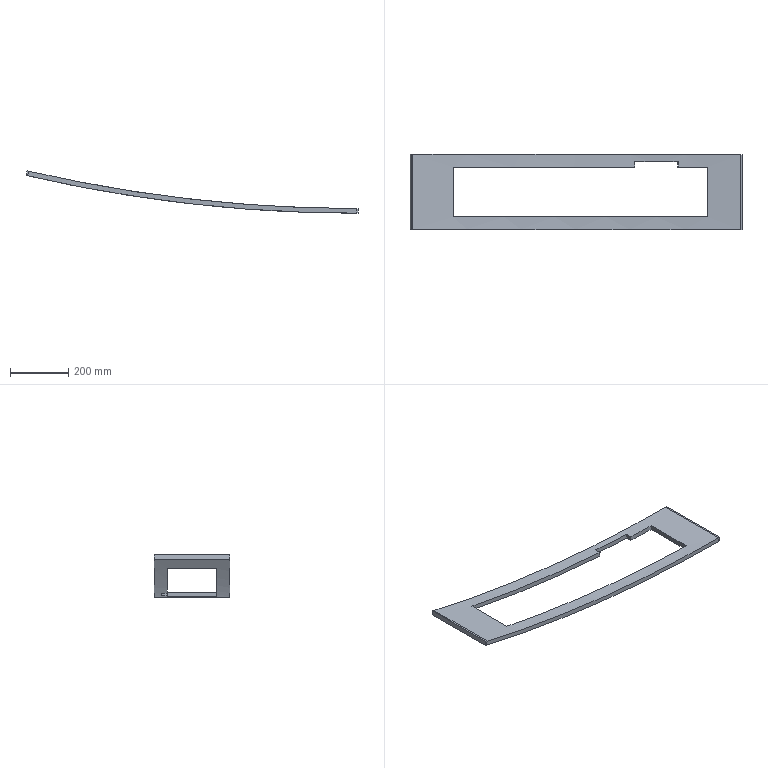Part | SolidWorks | features FlatPattern 1, SM3dBend 1, SMBaseFlange 1, SheetMetal 1 | 1 solid | 22 faces | box 1142 x 258 x 145.694 mm | volume 2305600 mm3 | plane 20 | cylinder 2 | commonest cylinder face diameters 10020 x1 10052 x1
STEP:
#1=CARTESIAN_POINT('',(17.269,258.,128.406));
#2=VERTEX_POINT('',#1);
#3=CARTESIAN_POINT('',(11.69,258.,129.694));
#4=VERTEX_POINT('',#3);
#5=CARTESIAN_POINT('',(11.69,258.,129.694));
#6=DIRECTION('',(-0.9744,0.,0.225));
#7=VECTOR('',#6,1000.);
#8=LINE('',#5,#7);
#9=EDGE_CURVE('',#2,#4,#8,.T.);
#10=ORIENTED_EDGE('',*,*,#9,.F.);
#11=CARTESIAN_POINT('',(13.67,258.,112.816));
#12=VERTEX_POINT('',#11);
#13=CARTESIAN_POINT('',(13.67,258.,112.816));
#14=DIRECTION('',(-0.225,0.,-0.9744));
#15=VECTOR('',#14,1000.);
#16=LINE('',#13,#15);
#17=EDGE_CURVE('',#2,#12,#16,.T.);
#18=ORIENTED_EDGE('',*,*,#17,.T.);
#19=CARTESIAN_POINT('',(8.091,258.,114.104));
#20=VERTEX_POINT('',#19);
#21=CARTESIAN_POINT('',(8.091,258.,114.104));
#22=DIRECTION('',(-0.9744,0.,0.225));
#23=VECTOR('',#22,1000.);
#24=LINE('',#21,#23);
#25=EDGE_CURVE('',#12,#20,#24,.T.);
#26=ORIENTED_EDGE('',*,*,#25,.T.);
#27=CARTESIAN_POINT('',(8.091,258.,114.104));
#28=DIRECTION('',(0.225,0.,0.9744));
#29=VECTOR('',#28,1000.);
#30=LINE('',#27,#29);
#31=EDGE_CURVE('',#20,#4,#30,.T.);
#32=ORIENTED_EDGE('',*,*,#31,.T.);
#33=EDGE_LOOP('',(#10,#18,#26,#32));
#34=FACE_OUTER_BOUND('',#33,.T.);
#35=CARTESIAN_POINT('',(8.091,258.,114.104));
#36=DIRECTION('',(0.,1.,0.));
#37=DIRECTION('',(0.225,0.,0.9744));
#38=AXIS2_PLACEMENT_3D('',#35,#36,#37);
#39=PLANE('',#38);
#40=ADVANCED_FACE('',(#34),#39,.T.);
#41=CARTESIAN_POINT('',(8.091,0.,114.104));
#42=VERTEX_POINT('',#41);
#43=CARTESIAN_POINT('',(13.67,0.,112.816));
#44=VERTEX_POINT('',#43);
#45=CARTESIAN_POINT('',(8.091,0.,114.104));
#46=DIRECTION('',(0.9744,0.,-0.225));
#47=VECTOR('',#46,1000.);
#48=LINE('',#45,#47);
#49=EDGE_CURVE('',#42,#44,#48,.T.);
#50=ORIENTED_EDGE('',*,*,#49,.T.);
#51=CARTESIAN_POINT('',(17.269,0.,128.406));
#52=VERTEX_POINT('',#51);
#53=CARTESIAN_POINT('',(13.67,0.,112.816));
#54=DIRECTION('',(0.225,0.,0.9744));
#55=VECTOR('',#54,1000.);
#56=LINE('',#53,#55);
#57=EDGE_CURVE('',#44,#52,#56,.T.);
#58=ORIENTED_EDGE('',*,*,#57,.T.);
#59=CARTESIAN_POINT('',(11.69,0.,129.694));
#60=VERTEX_POINT('',#59);
#61=CARTESIAN_POINT('',(11.69,0.,129.694));
#62=DIRECTION('',(0.9744,0.,-0.225));
#63=VECTOR('',#62,1000.);
#64=LINE('',#61,#63);
#65=EDGE_CURVE('',#60,#52,#64,.T.);
#66=ORIENTED_EDGE('',*,*,#65,.F.);
#67=CARTESIAN_POINT('',(8.091,0.,114.104));
#68=DIRECTION('',(0.225,0.,0.9744));
#69=VECTOR('',#68,1000.);
#70=LINE('',#67,#69);
#71=EDGE_CURVE('',#42,#60,#70,.T.);
#72=ORIENTED_EDGE('',*,*,#71,.F.);
#73=EDGE_LOOP('',(#50,#58,#66,#72));
#74=FACE_OUTER_BOUND('',#73,.T.);
#75=CARTESIAN_POINT('',(8.091,0.,114.104));
#76=DIRECTION('',(0.,-1.,0.));
#77=DIRECTION('',(-0.225,0.,-0.9744));
#78=AXIS2_PLACEMENT_3D('',#75,#76,#77);
#79=PLANE('',#78);
#80=ADVANCED_FACE('',(#74),#79,.T.);
#81=ORIENTED_EDGE('',*,*,#25,.F.);
#82=CARTESIAN_POINT('',(13.67,258.,112.816));
#83=DIRECTION('',(0.,-1.,0.));
#84=VECTOR('',#83,1000.);
#85=LINE('',#82,#84);
#86=EDGE_CURVE('',#12,#44,#85,.T.);
#87=ORIENTED_EDGE('',*,*,#86,.T.);
#88=ORIENTED_EDGE('',*,*,#49,.F.);
#89=CARTESIAN_POINT('',(8.091,0.,114.104));
#90=DIRECTION('',(0.,-1.,0.));
#91=VECTOR('',#90,1000.);
#92=LINE('',#89,#91);
#93=EDGE_CURVE('',#20,#42,#92,.T.);
#94=ORIENTED_EDGE('',*,*,#93,.F.);
#95=EDGE_LOOP('',(#81,#87,#88,#94));
#96=FACE_OUTER_BOUND('',#95,.T.);
#97=CARTESIAN_POINT('',(8.091,258.,114.104));
#98=DIRECTION('',(-0.225,0.,-0.9744));
#99=DIRECTION('',(-0.9744,0.,0.225));
#100=AXIS2_PLACEMENT_3D('',#97,#98,#99);
#101=PLANE('',#100);
#102=ADVANCED_FACE('',(#96),#101,.T.);
#103=CARTESIAN_POINT('',(11.69,0.,129.694));
#104=DIRECTION('',(0.,-1.,0.));
#105=VECTOR('',#104,1000.);
#106=LINE('',#103,#105);
#107=EDGE_CURVE('',#4,#60,#106,.T.);
#108=ORIENTED_EDGE('',*,*,#107,.F.);
#109=ORIENTED_EDGE('',*,*,#31,.F.);
#110=ORIENTED_EDGE('',*,*,#93,.T.);
#111=ORIENTED_EDGE('',*,*,#71,.T.);
#112=EDGE_LOOP('',(#108,#109,#110,#111));
#113=FACE_OUTER_BOUND('',#112,.T.);
#114=CARTESIAN_POINT('',(8.091,0.,114.104));
#115=DIRECTION('',(-0.9744,0.,0.225));
#116=DIRECTION('',(0.225,0.,0.9744));
#117=AXIS2_PLACEMENT_3D('',#114,#115,#116);
#118=PLANE('',#117);
#119=ADVANCED_FACE('',(#113),#118,.T.);
#120=CARTESIAN_POINT('',(17.269,258.,128.406));
#121=DIRECTION('',(0.,-1.,0.));
#122=VECTOR('',#121,1000.);
#123=LINE('',#120,#122);
#124=EDGE_CURVE('',#2,#52,#123,.T.);
#125=ORIENTED_EDGE('',*,*,#124,.F.);
#126=ORIENTED_EDGE('',*,*,#9,.T.);
#127=ORIENTED_EDGE('',*,*,#107,.T.);
#128=ORIENTED_EDGE('',*,*,#65,.T.);
#129=EDGE_LOOP('',(#125,#126,#127,#128));
#130=FACE_OUTER_BOUND('',#129,.T.);
#131=CARTESIAN_POINT('',(11.69,258.,129.694));
#132=DIRECTION('',(-0.225,0.,-0.9744));
#133=DIRECTION('',(-0.9744,0.,0.225));
#134=AXIS2_PLACEMENT_3D('',#131,#132,#133);
#135=PLANE('',#134);
#136=ADVANCED_FACE('',(#130),#135,.F.);
#137=CARTESIAN_POINT('',(1150.,0.,0.));
#138=VERTEX_POINT('',#137);
#139=CARTESIAN_POINT('',(1150.,258.,0.));
#140=VERTEX_POINT('',#139);
#141=CARTESIAN_POINT('',(1150.,0.,0.));
#142=DIRECTION('',(0.,1.,0.));
#143=VECTOR('',#142,1000.);
#144=LINE('',#141,#143);
#145=EDGE_CURVE('',#138,#140,#144,.T.);
#146=ORIENTED_EDGE('',*,*,#145,.F.);
#147=CARTESIAN_POINT('',(1150.,0.,-16.));
#148=VERTEX_POINT('',#147);
#149=CARTESIAN_POINT('',(1150.,0.,-16.));
#150=DIRECTION('',(0.,0.,1.));
#151=VECTOR('',#150,1000.);
#152=LINE('',#149,#151);
#153=EDGE_CURVE('',#148,#138,#152,.T.);
#154=ORIENTED_EDGE('',*,*,#153,.F.);
#155=CARTESIAN_POINT('',(1150.,258.,-16.));
#156=VERTEX_POINT('',#155);
#157=CARTESIAN_POINT('',(1150.,0.,-16.));
#158=DIRECTION('',(0.,1.,0.));
#159=VECTOR('',#158,1000.);
#160=LINE('',#157,#159);
#161=EDGE_CURVE('',#148,#156,#160,.T.);
#162=ORIENTED_EDGE('',*,*,#161,.T.);
#163=CARTESIAN_POINT('',(1150.,258.,-16.));
#164=DIRECTION('',(0.,0.,1.));
#165=VECTOR('',#164,1000.);
#166=LINE('',#163,#165);
#167=EDGE_CURVE('',#156,#140,#166,.T.);
#168=ORIENTED_EDGE('',*,*,#167,.T.);
#169=EDGE_LOOP('',(#146,#154,#162,#168));
#170=FACE_OUTER_BOUND('',#169,.T.);
#171=CARTESIAN_POINT('',(1150.,0.,-16.));
#172=DIRECTION('',(1.,0.,0.));
#173=DIRECTION('',(0.,0.,-1.));
#174=AXIS2_PLACEMENT_3D('',#171,#172,#173);
#175=PLANE('',#174);
#176=ADVANCED_FACE('',(#170),#175,.T.);
#177=CARTESIAN_POINT('',(1144.274,258.,-16.));
#178=VERTEX_POINT('',#177);
#179=CARTESIAN_POINT('',(1144.274,0.,-16.));
#180=VERTEX_POINT('',#179);
#181=CARTESIAN_POINT('',(1144.274,258.,-16.));
#182=DIRECTION('',(0.,-1.,0.));
#183=VECTOR('',#182,1000.);
#184=LINE('',#181,#183);
#185=EDGE_CURVE('',#178,#180,#184,.T.);
#186=ORIENTED_EDGE('',*,*,#185,.F.);
#187=CARTESIAN_POINT('',(0.,258.,-16.));
#188=DIRECTION('',(-1.,0.,0.));
#189=VECTOR('',#188,1000.);
#190=LINE('',#187,#189);
#191=EDGE_CURVE('',#156,#178,#190,.T.);
#192=ORIENTED_EDGE('',*,*,#191,.F.);
#193=ORIENTED_EDGE('',*,*,#161,.F.);
#194=CARTESIAN_POINT('',(0.,0.,-16.));
#195=DIRECTION('',(1.,0.,0.));
#196=VECTOR('',#195,1000.);
#197=LINE('',#194,#196);
#198=EDGE_CURVE('',#180,#148,#197,.T.);
#199=ORIENTED_EDGE('',*,*,#198,.F.);
#200=EDGE_LOOP('',(#186,#192,#193,#199));
#201=FACE_OUTER_BOUND('',#200,.T.);
#202=CARTESIAN_POINT('',(0.,258.,-16.));
#203=DIRECTION('',(0.,0.,-1.));
#204=DIRECTION('',(-1.,0.,0.));
#205=AXIS2_PLACEMENT_3D('',#202,#203,#204);
#206=PLANE('',#205);
#207=ADVANCED_FACE('',(#201),#206,.T.);
#208=CARTESIAN_POINT('',(1144.274,258.,0.));
#209=VERTEX_POINT('',#208);
#210=CARTESIAN_POINT('',(1144.274,258.,-16.));
#211=DIRECTION('',(0.,0.,-1.));
#212=VECTOR('',#211,1000.);
#213=LINE('',#210,#212);
#214=EDGE_CURVE('',#209,#178,#213,.T.);
#215=ORIENTED_EDGE('',*,*,#214,.F.);
#216=CARTESIAN_POINT('',(0.,258.,0.));
#217=DIRECTION('',(-1.,0.,0.));
#218=VECTOR('',#217,1000.);
#219=LINE('',#216,#218);
#220=EDGE_CURVE('',#140,#209,#219,.T.);
#221=ORIENTED_EDGE('',*,*,#220,.F.);
#222=ORIENTED_EDGE('',*,*,#167,.F.);
#223=ORIENTED_EDGE('',*,*,#191,.T.);
#224=EDGE_LOOP('',(#215,#221,#222,#223));
#225=FACE_OUTER_BOUND('',#224,.T.);
#226=CARTESIAN_POINT('',(0.,258.,-16.));
#227=DIRECTION('',(0.,1.,0.));
#228=DIRECTION('',(0.,0.,1.));
#229=AXIS2_PLACEMENT_3D('',#226,#227,#228);
#230=PLANE('',#229);
#231=ADVANCED_FACE('',(#225),#230,.T.);
#232=ORIENTED_EDGE('',*,*,#220,.T.);
#233=CARTESIAN_POINT('',(1144.274,0.,0.));
#234=VERTEX_POINT('',#233);
#235=CARTESIAN_POINT('',(1144.274,258.,0.));
#236=DIRECTION('',(0.,-1.,0.));
#237=VECTOR('',#236,1000.);
#238=LINE('',#235,#237);
#239=EDGE_CURVE('',#209,#234,#238,.T.);
#240=ORIENTED_EDGE('',*,*,#239,.T.);
#241=CARTESIAN_POINT('',(0.,0.,0.));
#242=DIRECTION('',(1.,0.,0.));
#243=VECTOR('',#242,1000.);
#244=LINE('',#241,#243);
#245=EDGE_CURVE('',#234,#138,#244,.T.);
#246=ORIENTED_EDGE('',*,*,#245,.T.);
#247=ORIENTED_EDGE('',*,*,#145,.T.);
#248=EDGE_LOOP('',(#232,#240,#246,#247));
#249=FACE_OUTER_BOUND('',#248,.T.);
#250=CARTESIAN_POINT('',(0.,258.,0.));
#251=DIRECTION('',(0.,0.,-1.));
#252=DIRECTION('',(-1.,0.,0.));
#253=AXIS2_PLACEMENT_3D('',#250,#251,#252);
#254=PLANE('',#253);
#255=ADVANCED_FACE('',(#249),#254,.F.);
#256=CARTESIAN_POINT('',(1144.274,0.,-16.));
#257=DIRECTION('',(0.,0.,1.));
#258=VECTOR('',#257,1000.);
#259=LINE('',#256,#258);
#260=EDGE_CURVE('',#180,#234,#259,.T.);
#261=ORIENTED_EDGE('',*,*,#260,.F.);
#262=ORIENTED_EDGE('',*,*,#198,.T.);
#263=ORIENTED_EDGE('',*,*,#153,.T.);
#264=ORIENTED_EDGE('',*,*,#245,.F.);
#265=EDGE_LOOP('',(#261,#262,#263,#264));
#266=FACE_OUTER_BOUND('',#265,.T.);
#267=CARTESIAN_POINT('',(0.,0.,-16.));
#268=DIRECTION('',(0.,-1.,0.));
#269=DIRECTION('',(0.,0.,-1.));
#270=AXIS2_PLACEMENT_3D('',#267,#268,#269);
#271=PLANE('',#270);
#272=ADVANCED_FACE('',(#266),#271,.T.);
#273=CARTESIAN_POINT('',(780.9,234.,13.195));
#274=VERTEX_POINT('',#273);
#275=CARTESIAN_POINT('',(779.74,234.,-2.763));
#276=VERTEX_POINT('',#275);
#277=CARTESIAN_POINT('',(779.74,234.,-2.763));
#278=DIRECTION('',(-0.07253,0.,-0.9974));
#279=VECTOR('',#278,1000.);
#280=LINE('',#277,#279);
#281=EDGE_CURVE('',#274,#276,#280,.T.);
#282=ORIENTED_EDGE('',*,*,#281,.F.);
#283=CARTESIAN_POINT('',(780.9,214.,13.195));
#284=VERTEX_POINT('',#283);
#285=CARTESIAN_POINT('',(780.9,-1038.524,13.195));
#286=DIRECTION('',(0.,-1.,0.));
#287=VECTOR('',#286,1000.);
#288=LINE('',#285,#287);
#289=EDGE_CURVE('',#274,#284,#288,.T.);
#290=ORIENTED_EDGE('',*,*,#289,.T.);
#291=CARTESIAN_POINT('',(779.74,214.,-2.763));
#292=VERTEX_POINT('',#291);
#293=CARTESIAN_POINT('',(779.74,214.,-2.763));
#294=DIRECTION('',(-0.07253,0.,-0.9974));
#295=VECTOR('',#294,1000.);
#296=LINE('',#293,#295);
#297=EDGE_CURVE('',#284,#292,#296,.T.);
#298=ORIENTED_EDGE('',*,*,#297,.T.);
#299=CARTESIAN_POINT('',(779.74,234.,-2.763));
#300=DIRECTION('',(0.,-1.,0.));
#301=VECTOR('',#300,1000.);
#302=LINE('',#299,#301);
#303=EDGE_CURVE('',#276,#292,#302,.T.);
#304=ORIENTED_EDGE('',*,*,#303,.F.);
#305=EDGE_LOOP('',(#282,#290,#298,#304));
#306=FACE_OUTER_BOUND('',#305,.T.);
#307=CARTESIAN_POINT('',(779.74,224.,-2.763));
#308=DIRECTION('',(0.9974,0.,-0.07253));
#309=DIRECTION('',(0.,-1.,0.));
#310=AXIS2_PLACEMENT_3D('',#307,#308,#309);
#311=PLANE('',#310);
#312=ADVANCED_FACE('',(#306),#311,.T.);
#313=ORIENTED_EDGE('',*,*,#297,.F.);
#314=CARTESIAN_POINT('',(158.068,214.,98.025));
#315=VERTEX_POINT('',#314);
#316=CARTESIAN_POINT('',(1144.274,214.,5010.));
#317=DIRECTION('',(0.,1.,0.));
#318=DIRECTION('',(0.,0.,1.));
#319=AXIS2_PLACEMENT_3D('',#316,#317,#318);
#320=CIRCLE('',#319,5010.);
#321=EDGE_CURVE('',#284,#315,#320,.T.);
#322=ORIENTED_EDGE('',*,*,#321,.T.);
#323=CARTESIAN_POINT('',(154.918,214.,82.338));
#324=VERTEX_POINT('',#323);
#325=CARTESIAN_POINT('',(154.918,214.,82.338));
#326=DIRECTION('',(-0.1968,0.,-0.9804));
#327=VECTOR('',#326,1000.);
#328=LINE('',#325,#327);
#329=EDGE_CURVE('',#315,#324,#328,.T.);
#330=ORIENTED_EDGE('',*,*,#329,.T.);
#331=CARTESIAN_POINT('',(1144.274,214.,5010.));
#332=DIRECTION('',(0.,1.,0.));
#333=DIRECTION('',(0.,0.,1.));
#334=AXIS2_PLACEMENT_3D('',#331,#332,#333);
#335=CIRCLE('',#334,5026.);
#336=EDGE_CURVE('',#292,#324,#335,.T.);
#337=ORIENTED_EDGE('',*,*,#336,.F.);
#338=EDGE_LOOP('',(#313,#322,#330,#337));
#339=FACE_OUTER_BOUND('',#338,.T.);
#340=CARTESIAN_POINT('',(1144.274,214.,5010.));
#341=DIRECTION('',(0.,-1.,0.));
#342=DIRECTION('',(0.,0.,-1.));
#343=AXIS2_PLACEMENT_3D('',#340,#341,#342);
#344=PLANE('',#343);
#345=ADVANCED_FACE('',(#339),#344,.T.);
#346=ORIENTED_EDGE('',*,*,#329,.F.);
#347=CARTESIAN_POINT('',(158.068,44.,98.025));
#348=VERTEX_POINT('',#347);
#349=CARTESIAN_POINT('',(158.068,-1038.524,98.025));
#350=DIRECTION('',(0.,-1.,0.));
#351=VECTOR('',#350,1000.);
#352=LINE('',#349,#351);
#353=EDGE_CURVE('',#315,#348,#352,.T.);
#354=ORIENTED_EDGE('',*,*,#353,.T.);
#355=CARTESIAN_POINT('',(154.918,44.,82.338));
#356=VERTEX_POINT('',#355);
#357=CARTESIAN_POINT('',(154.918,44.,82.338));
#358=DIRECTION('',(-0.1968,0.,-0.9804));
#359=VECTOR('',#358,1000.);
#360=LINE('',#357,#359);
#361=EDGE_CURVE('',#348,#356,#360,.T.);
#362=ORIENTED_EDGE('',*,*,#361,.T.);
#363=CARTESIAN_POINT('',(154.918,214.,82.338));
#364=DIRECTION('',(0.,-1.,0.));
#365=VECTOR('',#364,1000.);
#366=LINE('',#363,#365);
#367=EDGE_CURVE('',#324,#356,#366,.T.);
#368=ORIENTED_EDGE('',*,*,#367,.F.);
#369=EDGE_LOOP('',(#346,#354,#362,#368));
#370=FACE_OUTER_BOUND('',#369,.T.);
#371=CARTESIAN_POINT('',(154.918,129.,82.338));
#372=DIRECTION('',(0.9804,0.,-0.1968));
#373=DIRECTION('',(0.,-1.,0.));
#374=AXIS2_PLACEMENT_3D('',#371,#372,#373);
#375=PLANE('',#374);
#376=ADVANCED_FACE('',(#370),#375,.T.);
#377=ORIENTED_EDGE('',*,*,#361,.F.);
#378=CARTESIAN_POINT('',(1030.192,44.,1.299));
#379=VERTEX_POINT('',#378);
#380=CARTESIAN_POINT('',(1144.274,44.,5010.));
#381=DIRECTION('',(0.,-1.,0.));
#382=DIRECTION('',(0.,0.,1.));
#383=AXIS2_PLACEMENT_3D('',#380,#381,#382);
#384=CIRCLE('',#383,5010.);
#385=EDGE_CURVE('',#348,#379,#384,.T.);
#386=ORIENTED_EDGE('',*,*,#385,.T.);
#387=CARTESIAN_POINT('',(1029.828,44.,-14.697));
#388=VERTEX_POINT('',#387);
#389=CARTESIAN_POINT('',(1029.828,44.,-14.697));
#390=DIRECTION('',(-0.02277,0.,-0.9997));
#391=VECTOR('',#390,1000.);
#392=LINE('',#389,#391);
#393=EDGE_CURVE('',#379,#388,#392,.T.);
#394=ORIENTED_EDGE('',*,*,#393,.T.);
#395=CARTESIAN_POINT('',(1144.274,44.,5010.));
#396=DIRECTION('',(0.,-1.,0.));
#397=DIRECTION('',(0.,0.,-1.));
#398=AXIS2_PLACEMENT_3D('',#395,#396,#397);
#399=CIRCLE('',#398,5026.);
#400=EDGE_CURVE('',#356,#388,#399,.T.);
#401=ORIENTED_EDGE('',*,*,#400,.F.);
#402=EDGE_LOOP('',(#377,#386,#394,#401));
#403=FACE_OUTER_BOUND('',#402,.T.);
#404=CARTESIAN_POINT('',(1144.274,44.,5010.));
#405=DIRECTION('',(0.,1.,0.));
#406=DIRECTION('',(0.,0.,1.));
#407=AXIS2_PLACEMENT_3D('',#404,#405,#406);
#408=PLANE('',#407);
#409=ADVANCED_FACE('',(#403),#408,.T.);
#410=ORIENTED_EDGE('',*,*,#393,.F.);
#411=CARTESIAN_POINT('',(1030.192,214.,1.299));
#412=VERTEX_POINT('',#411);
#413=CARTESIAN_POINT('',(1030.192,-1038.524,1.299));
#414=DIRECTION('',(0.,1.,0.));
#415=VECTOR('',#414,1000.);
#416=LINE('',#413,#415);
#417=EDGE_CURVE('',#379,#412,#416,.T.);
#418=ORIENTED_EDGE('',*,*,#417,.T.);
#419=CARTESIAN_POINT('',(1029.828,214.,-14.697));
#420=VERTEX_POINT('',#419);
#421=CARTESIAN_POINT('',(1029.828,214.,-14.697));
#422=DIRECTION('',(-0.02277,0.,-0.9997));
#423=VECTOR('',#422,1000.);
#424=LINE('',#421,#423);
#425=EDGE_CURVE('',#412,#420,#424,.T.);
#426=ORIENTED_EDGE('',*,*,#425,.T.);
#427=CARTESIAN_POINT('',(1029.828,44.,-14.697));
#428=DIRECTION('',(0.,1.,0.));
#429=VECTOR('',#428,1000.);
#430=LINE('',#427,#429);
#431=EDGE_CURVE('',#388,#420,#430,.T.);
#432=ORIENTED_EDGE('',*,*,#431,.F.);
#433=EDGE_LOOP('',(#410,#418,#426,#432));
#434=FACE_OUTER_BOUND('',#433,.T.);
#435=CARTESIAN_POINT('',(1029.828,129.,-14.697));
#436=DIRECTION('',(-0.9997,0.,0.02277));
#437=DIRECTION('',(0.,1.,0.));
#438=AXIS2_PLACEMENT_3D('',#435,#436,#437);
#439=PLANE('',#438);
#440=ADVANCED_FACE('',(#434),#439,.T.);
#441=ORIENTED_EDGE('',*,*,#425,.F.);
#442=CARTESIAN_POINT('',(930.407,214.,4.567));
#443=VERTEX_POINT('',#442);
#444=CARTESIAN_POINT('',(1144.274,214.,5010.));
#445=DIRECTION('',(0.,1.,0.));
#446=DIRECTION('',(0.,0.,1.));
#447=AXIS2_PLACEMENT_3D('',#444,#445,#446);
#448=CIRCLE('',#447,5010.);
#449=EDGE_CURVE('',#412,#443,#448,.T.);
#450=ORIENTED_EDGE('',*,*,#449,.T.);
#451=CARTESIAN_POINT('',(929.724,214.,-11.419));
#452=VERTEX_POINT('',#451);
#453=CARTESIAN_POINT('',(929.724,214.,-11.419));
#454=DIRECTION('',(-0.04269,0.,-0.9991));
#455=VECTOR('',#454,1000.);
#456=LINE('',#453,#455);
#457=EDGE_CURVE('',#443,#452,#456,.T.);
#458=ORIENTED_EDGE('',*,*,#457,.T.);
#459=CARTESIAN_POINT('',(1144.274,214.,5010.));
#460=DIRECTION('',(0.,1.,0.));
#461=DIRECTION('',(0.,0.,1.));
#462=AXIS2_PLACEMENT_3D('',#459,#460,#461);
#463=CIRCLE('',#462,5026.);
#464=EDGE_CURVE('',#420,#452,#463,.T.);
#465=ORIENTED_EDGE('',*,*,#464,.F.);
#466=EDGE_LOOP('',(#441,#450,#458,#465));
#467=FACE_OUTER_BOUND('',#466,.T.);
#468=CARTESIAN_POINT('',(1144.274,214.,5010.));
#469=DIRECTION('',(0.,-1.,0.));
#470=DIRECTION('',(0.,0.,-1.));
#471=AXIS2_PLACEMENT_3D('',#468,#469,#470);
#472=PLANE('',#471);
#473=ADVANCED_FACE('',(#467),#472,.T.);
#474=ORIENTED_EDGE('',*,*,#457,.F.);
#475=CARTESIAN_POINT('',(930.407,234.,4.567));
#476=VERTEX_POINT('',#475);
#477=CARTESIAN_POINT('',(930.407,-1038.524,4.567));
#478=DIRECTION('',(0.,1.,0.));
#479=VECTOR('',#478,1000.);
#480=LINE('',#477,#479);
#481=EDGE_CURVE('',#443,#476,#480,.T.);
#482=ORIENTED_EDGE('',*,*,#481,.T.);
#483=CARTESIAN_POINT('',(929.724,234.,-11.419));
#484=VERTEX_POINT('',#483);
#485=CARTESIAN_POINT('',(929.724,234.,-11.419));
#486=DIRECTION('',(-0.04269,0.,-0.9991));
#487=VECTOR('',#486,1000.);
#488=LINE('',#485,#487);
#489=EDGE_CURVE('',#476,#484,#488,.T.);
#490=ORIENTED_EDGE('',*,*,#489,.T.);
#491=CARTESIAN_POINT('',(929.724,214.,-11.419));
#492=DIRECTION('',(0.,1.,0.));
#493=VECTOR('',#492,1000.);
#494=LINE('',#491,#493);
#495=EDGE_CURVE('',#452,#484,#494,.T.);
#496=ORIENTED_EDGE('',*,*,#495,.F.);
#497=EDGE_LOOP('',(#474,#482,#490,#496));
#498=FACE_OUTER_BOUND('',#497,.T.);
#499=CARTESIAN_POINT('',(929.724,224.,-11.419));
#500=DIRECTION('',(-0.9991,0.,0.04269));
#501=DIRECTION('',(0.,1.,0.));
#502=AXIS2_PLACEMENT_3D('',#499,#500,#501);
#503=PLANE('',#502);
#504=ADVANCED_FACE('',(#498),#503,.T.);
#505=ORIENTED_EDGE('',*,*,#17,.F.);
#506=CARTESIAN_POINT('',(1144.274,258.,5010.));
#507=DIRECTION('',(0.,-1.,0.));
#508=DIRECTION('',(0.,0.,1.));
#509=AXIS2_PLACEMENT_3D('',#506,#507,#508);
#510=CIRCLE('',#509,5010.);
#511=EDGE_CURVE('',#2,#209,#510,.T.);
#512=ORIENTED_EDGE('',*,*,#511,.T.);
#513=ORIENTED_EDGE('',*,*,#214,.T.);
#514=CARTESIAN_POINT('',(1144.274,258.,5010.));
#515=DIRECTION('',(0.,-1.,0.));
#516=DIRECTION('',(0.,0.,1.));
#517=AXIS2_PLACEMENT_3D('',#514,#515,#516);
#518=CIRCLE('',#517,5026.);
#519=EDGE_CURVE('',#12,#178,#518,.T.);
#520=ORIENTED_EDGE('',*,*,#519,.F.);
#521=EDGE_LOOP('',(#505,#512,#513,#520));
#522=FACE_OUTER_BOUND('',#521,.T.);
#523=CARTESIAN_POINT('',(1144.274,258.,5010.));
#524=DIRECTION('',(0.,1.,0.));
#525=DIRECTION('',(0.,0.,1.));
#526=AXIS2_PLACEMENT_3D('',#523,#524,#525);
#527=PLANE('',#526);
#528=ADVANCED_FACE('',(#522),#527,.T.);
#529=ORIENTED_EDGE('',*,*,#185,.T.);
#530=CARTESIAN_POINT('',(1144.274,0.,5010.));
#531=DIRECTION('',(0.,1.,0.));
#532=DIRECTION('',(0.,0.,-1.));
#533=AXIS2_PLACEMENT_3D('',#530,#531,#532);
#534=CIRCLE('',#533,5026.);
#535=EDGE_CURVE('',#180,#44,#534,.T.);
#536=ORIENTED_EDGE('',*,*,#535,.T.);
#537=ORIENTED_EDGE('',*,*,#86,.F.);
#538=ORIENTED_EDGE('',*,*,#519,.T.);
#539=EDGE_LOOP('',(#529,#536,#537,#538));
#540=FACE_OUTER_BOUND('',#539,.T.);
#541=ORIENTED_EDGE('',*,*,#495,.T.);
#542=CARTESIAN_POINT('',(1144.274,234.,5010.));
#543=DIRECTION('',(0.,1.,0.));
#544=DIRECTION('',(0.,0.,1.));
#545=AXIS2_PLACEMENT_3D('',#542,#543,#544);
#546=CIRCLE('',#545,5026.);
#547=EDGE_CURVE('',#484,#276,#546,.T.);
#548=ORIENTED_EDGE('',*,*,#547,.T.);
#549=ORIENTED_EDGE('',*,*,#303,.T.);
#550=ORIENTED_EDGE('',*,*,#336,.T.);
#551=ORIENTED_EDGE('',*,*,#367,.T.);
#552=ORIENTED_EDGE('',*,*,#400,.T.);
#553=ORIENTED_EDGE('',*,*,#431,.T.);
#554=ORIENTED_EDGE('',*,*,#464,.T.);
#555=EDGE_LOOP('',(#541,#548,#549,#550,#551,#552,#553,#554));
#556=FACE_BOUND('',#555,.T.);
#557=CARTESIAN_POINT('',(1144.274,-1038.524,5010.));
#558=DIRECTION('',(0.,1.,0.));
#559=DIRECTION('',(0.,0.,1.));
#560=AXIS2_PLACEMENT_3D('',#557,#558,#559);
#561=CYLINDRICAL_SURFACE('',#560,5026.);
#562=ADVANCED_FACE('',(#540,#556),#561,.T.);
#563=CARTESIAN_POINT('',(1144.274,234.,5010.));
#564=DIRECTION('',(0.,1.,0.));
#565=DIRECTION('',(0.,0.,1.));
#566=AXIS2_PLACEMENT_3D('',#563,#564,#565);
#567=CIRCLE('',#566,5010.);
#568=EDGE_CURVE('',#476,#274,#567,.T.);
#569=ORIENTED_EDGE('',*,*,#568,.T.);
#570=ORIENTED_EDGE('',*,*,#281,.T.);
#571=ORIENTED_EDGE('',*,*,#547,.F.);
#572=ORIENTED_EDGE('',*,*,#489,.F.);
#573=EDGE_LOOP('',(#569,#570,#571,#572));
#574=FACE_OUTER_BOUND('',#573,.T.);
#575=CARTESIAN_POINT('',(1144.274,234.,5010.));
#576=DIRECTION('',(0.,-1.,0.));
#577=DIRECTION('',(0.,0.,-1.));
#578=AXIS2_PLACEMENT_3D('',#575,#576,#577);
#579=PLANE('',#578);
#580=ADVANCED_FACE('',(#574),#579,.T.);
#581=CARTESIAN_POINT('',(1144.274,0.,5010.));
#582=DIRECTION('',(0.,1.,0.));
#583=DIRECTION('',(0.,0.,1.));
#584=AXIS2_PLACEMENT_3D('',#581,#582,#583);
#585=CIRCLE('',#584,5010.);
#586=EDGE_CURVE('',#234,#52,#585,.T.);
#587=ORIENTED_EDGE('',*,*,#586,.T.);
#588=ORIENTED_EDGE('',*,*,#57,.F.);
#589=ORIENTED_EDGE('',*,*,#535,.F.);
#590=ORIENTED_EDGE('',*,*,#260,.T.);
#591=EDGE_LOOP('',(#587,#588,#589,#590));
#592=FACE_OUTER_BOUND('',#591,.T.);
#593=CARTESIAN_POINT('',(1144.274,0.,5010.));
#594=DIRECTION('',(0.,-1.,0.));
#595=DIRECTION('',(0.,0.,-1.));
#596=AXIS2_PLACEMENT_3D('',#593,#594,#595);
#597=PLANE('',#596);
#598=ADVANCED_FACE('',(#592),#597,.T.);
#599=ORIENTED_EDGE('',*,*,#239,.F.);
#600=ORIENTED_EDGE('',*,*,#511,.F.);
#601=ORIENTED_EDGE('',*,*,#124,.T.);
#602=ORIENTED_EDGE('',*,*,#586,.F.);
#603=EDGE_LOOP('',(#599,#600,#601,#602));
#604=FACE_OUTER_BOUND('',#603,.T.);
#605=ORIENTED_EDGE('',*,*,#481,.F.);
#606=ORIENTED_EDGE('',*,*,#449,.F.);
#607=ORIENTED_EDGE('',*,*,#417,.F.);
#608=ORIENTED_EDGE('',*,*,#385,.F.);
#609=ORIENTED_EDGE('',*,*,#353,.F.);
#610=ORIENTED_EDGE('',*,*,#321,.F.);
#611=ORIENTED_EDGE('',*,*,#289,.F.);
#612=ORIENTED_EDGE('',*,*,#568,.F.);
#613=EDGE_LOOP('',(#605,#606,#607,#608,#609,#610,#611,#612));
#614=FACE_BOUND('',#613,.T.);
#615=CARTESIAN_POINT('',(1144.274,-1038.524,5010.));
#616=DIRECTION('',(0.,1.,0.));
#617=DIRECTION('',(0.,0.,1.));
#618=AXIS2_PLACEMENT_3D('',#615,#616,#617);
#619=CYLINDRICAL_SURFACE('',#618,5010.);
#620=ADVANCED_FACE('',(#604,#614),#619,.F.);
#621=CLOSED_SHELL('',(#40,#80,#102,#119,#136,#176,#207,#231,#255,#272,#312,#345,#376,#409,#440,#473,#504,#528,#562,#580,#598,#620));
#622=MANIFOLD_SOLID_BREP('',#621);
#623=CARTESIAN_POINT('',(0.,0.,0.));
#624=DIRECTION('',(0.,0.,1.));
#625=DIRECTION('',(1.,0.,0.));
#626=AXIS2_PLACEMENT_3D('',#623,#624,#625);
#627=(LENGTH_UNIT()NAMED_UNIT(*)SI_UNIT(.MILLI.,.METRE.));
#628=UNCERTAINTY_MEASURE_WITH_UNIT(LENGTH_MEASURE(0.00001),#627,'','');
#629=(NAMED_UNIT(*)PLANE_ANGLE_UNIT()SI_UNIT($,.RADIAN.));
#630=(NAMED_UNIT(*)SI_UNIT($,.STERADIAN.)SOLID_ANGLE_UNIT());
#631=(GEOMETRIC_REPRESENTATION_CONTEXT(3)GLOBAL_UNCERTAINTY_ASSIGNED_CONTEXT((#628))GLOBAL_UNIT_ASSIGNED_CONTEXT((#627,#629,#630))REPRESENTATION_CONTEXT('',''));
#632=ADVANCED_BREP_SHAPE_REPRESENTATION('',(#622,#626),#631);